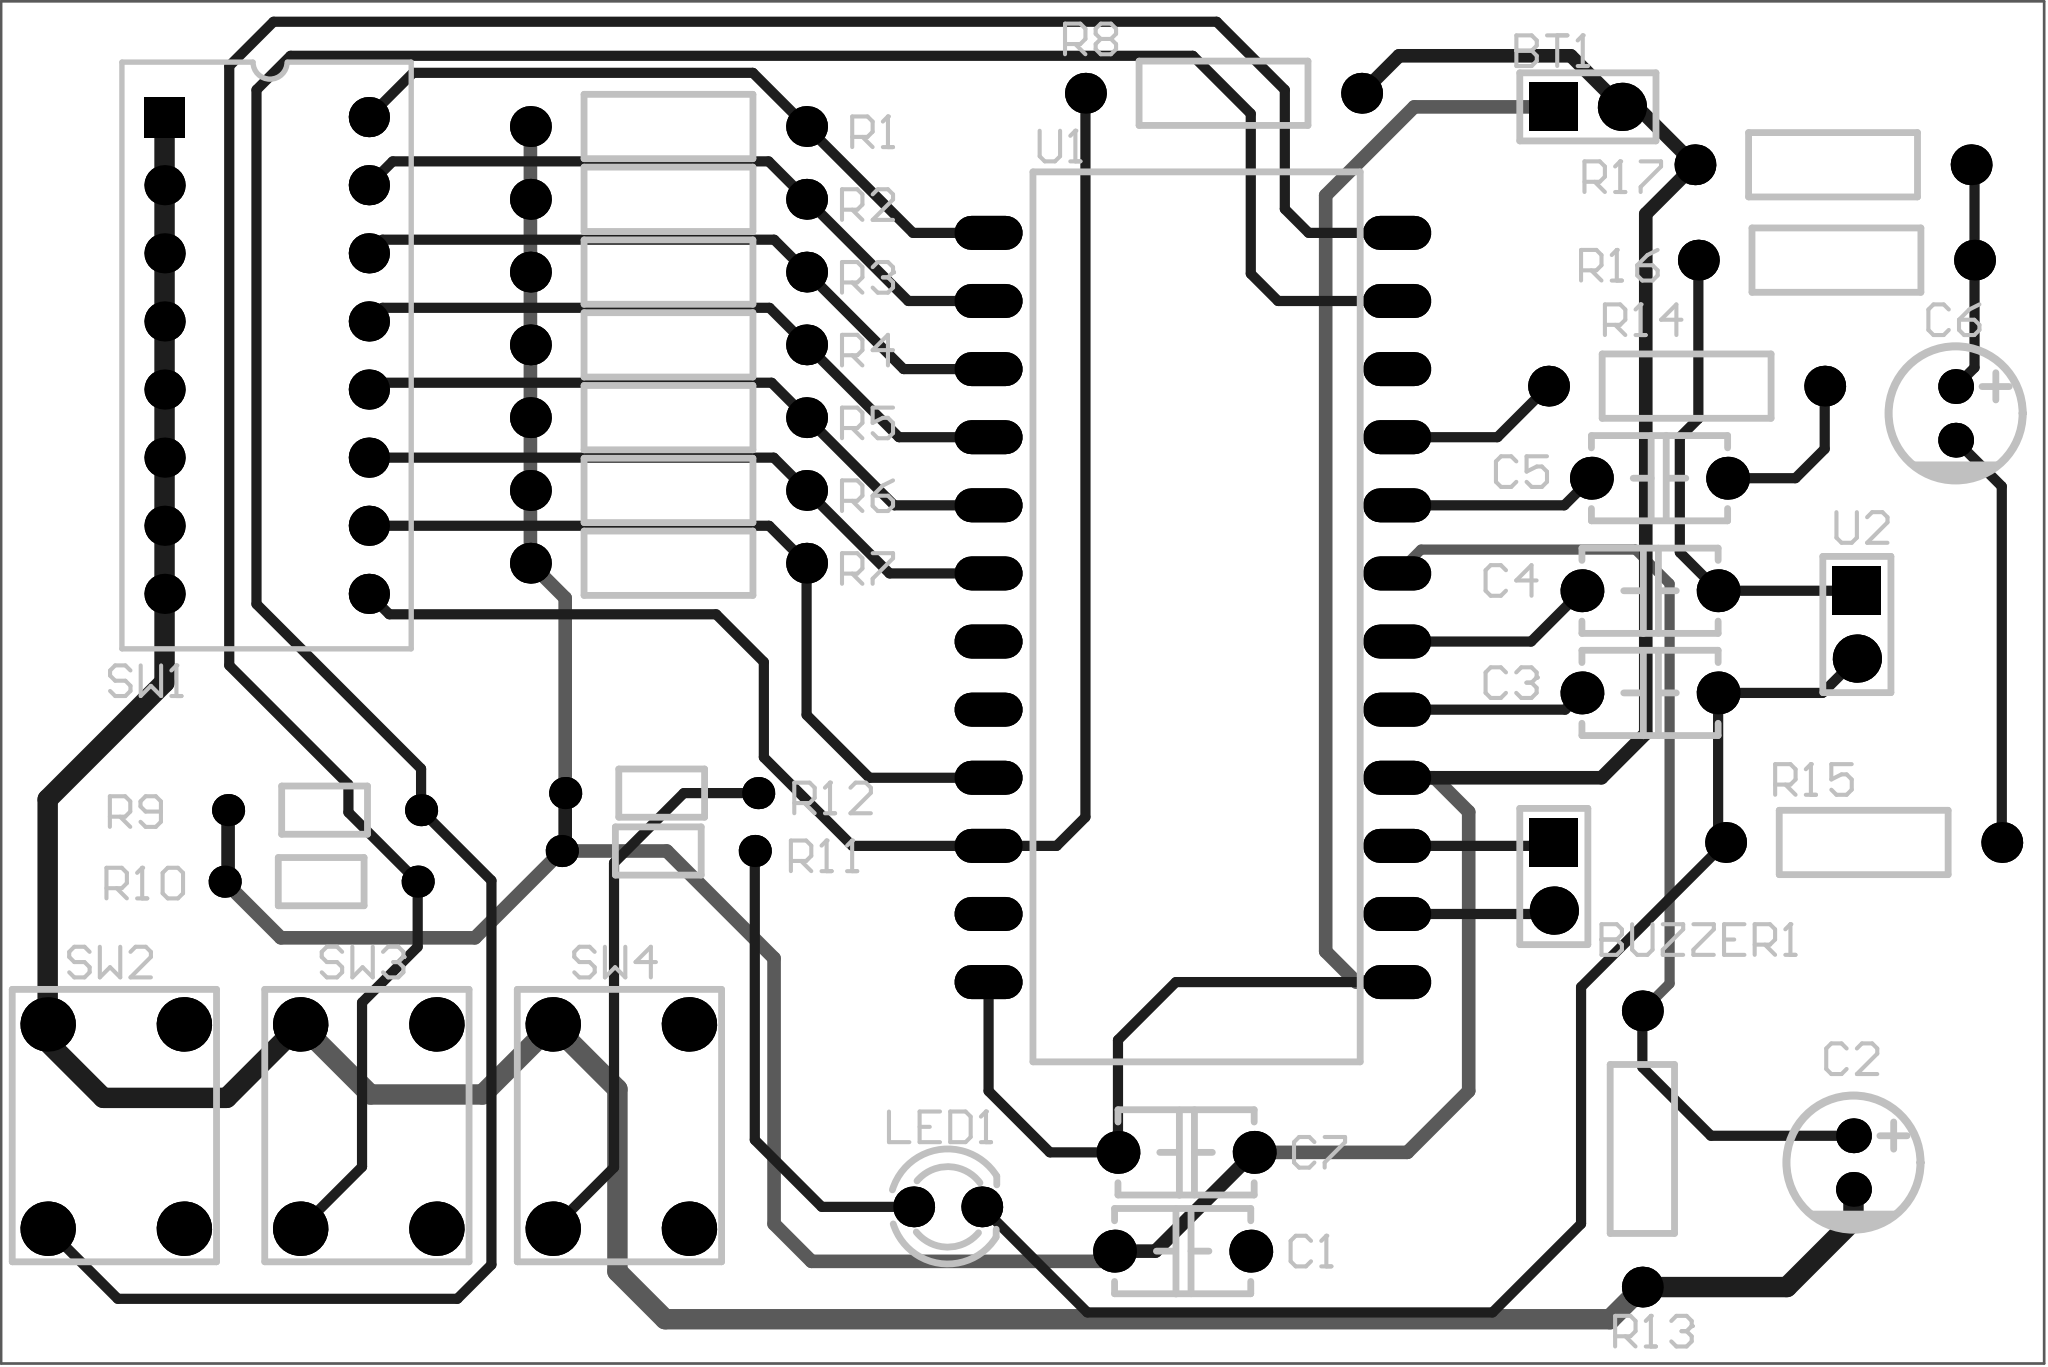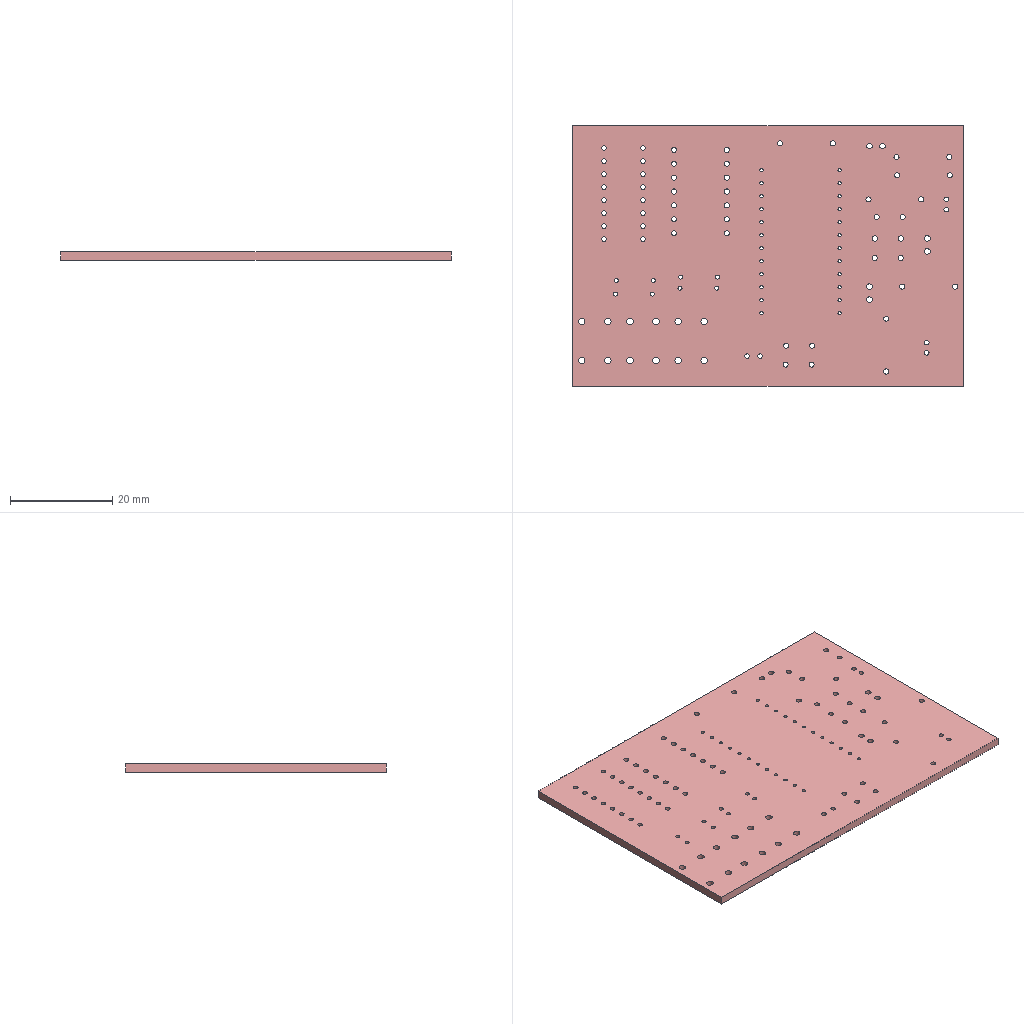Circuit board layout | Altium Designer | box 76.2 x 50.8 x 1.6 mm
Layer stack:
# Altium Designer layer stack of  (unit mm; dielectric type: 0 none, 1 core, 2 prepreg, 3 surface material)
index,name,kind,layer,copper_thickness_mm,dielectric_type,dielectric_thickness_mm,dielectric_material,dielectric_constant
0,Top Paste Mask Layer,other,,,,,,
1,Top Silkscreen Layer,other,,,,,,
2,Top Solder Mask Layer,dielectric,,,3,0.01,,3.3
3,Top Layer,copper,Top Layer,0.035,,,,
4,Dielectric1,dielectric,,,3,1.51,FR4,4.5
5,Bottom Layer,copper,Bottom Layer,0.035,,,,
6,Bottom Solder Mask Layer,dielectric,,,3,0.01,,3.3
7,Bottom Silkscreen Layer,other,,,,,,
8,Bottom Paste Mask Layer,other,,,,,,
# drill layer pairs: low layer,high layer
drill_pair,Top Layer,Bottom Layer
Part placement:
Designator,Comment,Layer,Footprint,Center-X(mm),Center-Y(mm),Rotation
BT1,,TopLayer,HDR-TH_2P-P2.54-V-M-1,138.217,123.063,0
BUZZER1,SPEAKER,TopLayer,HDR-TH_2P-P2.54-V-M-1,136.947,94.361,270
C1,0.0uF,TopLayer,CAP-TH_L5.1-W3.2-P5.08-D0.50,123.104,80.391,0
C2,4.7uF,TopLayer,CAP-TH_BD5.0-P2.00-D0.8-FD-10UF50VC110GL,148.123,83.693,270
C3,0.1uF,TopLayer,CAP-TH_L5.1-W3.2-P5.08-D0.50,140.535,101.208,0
C4,0.1uF,TopLayer,CAP-TH_L5.1-W3.2-P5.08-D0.50,140.535,105.018,0
C5,0.1uF,TopLayer,CAP-TH_L5.1-W3.2-P5.08-D0.50,140.889,109.215,180
C6,220uF,TopLayer,CAP-TH_BD5.0-P2.00-D0.8-FD-10UF50VC110GL,151.933,111.633,270
LED1,,TopLayer,LED_TH-3mm,114.341,82.042,0
R1,10kΩ,TopLayer,Res_1/4W,103.927,122.331,180
R2,10kΩ,TopLayer,Res_1/4W,103.927,119.617,180
R3,10kΩ,TopLayer,Res_1/4W,103.927,116.902,180
R4,10kΩ,TopLayer,Res_1/4W,103.927,114.188,180
R5,10kΩ,TopLayer,Res_1/4W,103.927,111.474,180
R6,10kΩ,TopLayer,Res_1/4W,103.927,108.759,180
R7,10kΩ,TopLayer,Res_1/4W,103.927,106.045,180
R8,10kΩ,TopLayer,Res_1/4W,124.628,123.571,0
R9,100kΩ,TopLayer,Res_1/8W,91.1,96.837,0
R10,100kΩ,TopLayer,Res_1/8W,90.973,94.17,0
R11,5.1kΩ,TopLayer,Res_1/8W,103.546,95.313,0
R12,100kΩ,TopLayer,Res_1/8W,103.673,97.472,0
R13,470kΩ,TopLayer,Res_1/4W,140.249,84.201,90
R14,5.1kΩ,TopLayer,Res_1/4W,141.9,112.649,180
R15,10kΩ,TopLayer,Res_1/4W,148.504,95.631,0
R16,10kΩ,TopLayer,Res_1/4W,147.488,117.348,0
R17,1kΩ,TopLayer,Res_1/4W,147.361,120.904,180
SW1,SW-DIP8,TopLayer,SW-DIP8,88.941,113.792,90
SW2,,TopLayer,SW-TH_4P-L6.0-W6.0-P4.50-LS6.5,83.312,85.037,0
SW3,,TopLayer,SW-TH_4P-L6.0-W6.0-P4.50-LS6.5,92.731,85.037,0
SW4,,TopLayer,SW-TH_4P-L6.0-W6.0-P4.50-LS6.5,102.149,85.037,0
U1,,TopLayer,DIP-24_L30.4-W12.7-P2.54-LS10.1-BL,123.485,104.394,270
U2,,TopLayer,HDR-TH_2P-P2.54-V-M-1,148.25,103.759,270
C7,0.1uF,TopLayer,CAP-TH_L5.1-W3.2-P5.08-D0.50,123.231,84.074,0
Pad and via stacks:
# Altium Designer via and pad stacks of  (unit mm). Each distinct definition once, with the count of objects using it.
# via: kind,start_layer,end_layer,hole_mm,diameter_mm,mode(0 simple;1 top-mid-bottom;2 full stack),diameter_per_layer,count,example_net
# pad: kind,layer,hole_mm,hole_type(0 round;1 square;2 slot),plating,top_size,top_shape(1 round;2 rect;3 octagon;9 rounded rect),mid_size,bottom_size,mode,footprint,size_per_layer,count,example
pad,Multi-Layer,1.1,0,plated,1.8x1.8,1,1.8x1.8,1.8x1.8,0,HDR-TH_2P-P2.54-V-M-1,,3,BT1.2
pad,Multi-Layer,1.1,0,plated,1.8x1.8,2,1.8x1.8,1.8x1.8,0,HDR-TH_2P-P2.54-V-M-1,,3,BT1.1
pad,Multi-Layer,1,0,plated,1.6x1.6,1,1.6x1.6,1.6x1.6,0,CAP-TH_L5.1-W3.2-P5.08-D0.50,,10,C1.2
pad,Multi-Layer,0.9,0,plated,1.3x1.3,1,1.3x1.3,1.3x1.3,0,CAP-TH_BD5.0-P2.00-D0.8-FD-10UF50VC110GL,,4,C2.2
pad,Multi-Layer,0.9144,0,plated,1.524x1.524,1,1.524x1.524,1.524x1.524,0,LED_TH-3mm,,2,LED1.1
pad,Multi-Layer,1,0,plated,1.524x1.524,1,1.524x1.524,1.524x1.524,0,Res_1/4W,,26,R1.1
pad,Multi-Layer,0.8001,0,plated,1.199x1.199,1,1.199x1.199,1.199x1.199,0,Res_1/8W,,8,R9.1
pad,Multi-Layer,0.9,0,plated,1.5x1.5,1,1.5x1.5,1.5x1.5,0,SW-DIP8,,15,SW1.3
pad,Multi-Layer,0.9,0,plated,1.5x1.5,2,1.5x1.5,1.5x1.5,0,SW-DIP8,,1,SW1.1
pad,Multi-Layer,1.27,0,plated,2.032x2.032,1,2.032x2.032,2.032x2.032,0,SW-TH_4P-L6.0-W6.0-P4.50-LS6.5,,12,SW2.1
pad,Multi-Layer,0.635,0,plated,1.27x2.54,1,1.27x2.54,1.27x2.54,0,DIP-24_L30.4-W12.7-P2.54-LS10.1-BL,,24,U1.1
Design rules, without the lines most boards share:
# Altium Designer design rules of  (exported by Altium Designer, unit mm)
# columns: name | kind | enabled | priority | scope1 | scope2 | descriptor | typed fields (field=value)
creepage | 65 | enabled | 1 | All | All | Creepage Distance Constraint =(0mil) (All),(All) |